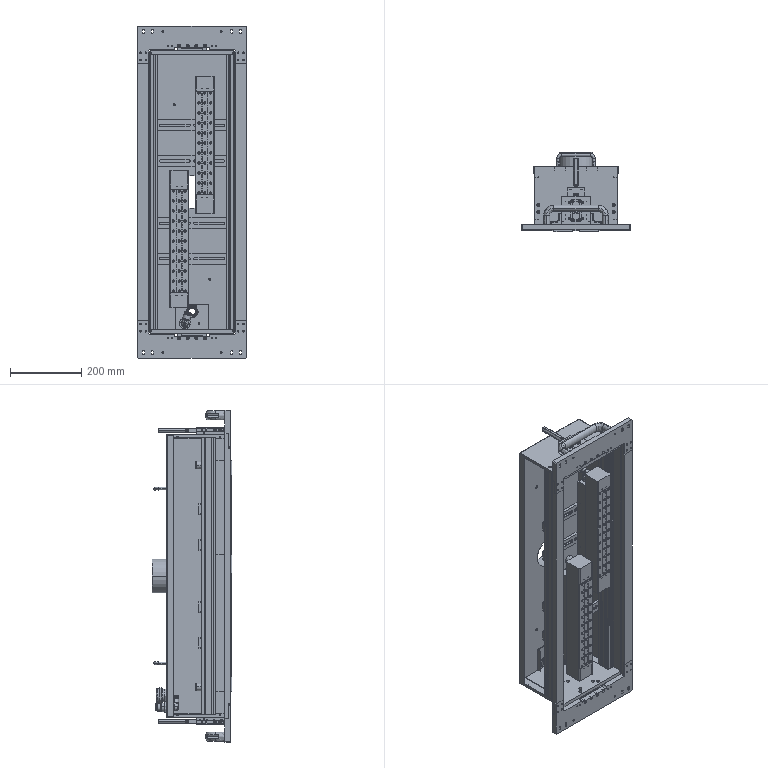Part | SolidWorks | 25 solids | 4655 faces | volume 6464827 mm3 | cylinder 2167 | plane 1377 | cone 986 | spline 51 | torus 44 | sphere 30 | commonest cylinder face diameters 1 x458 3.3 x210 8 x168 4.5 x142 0.659 x131 10 x118